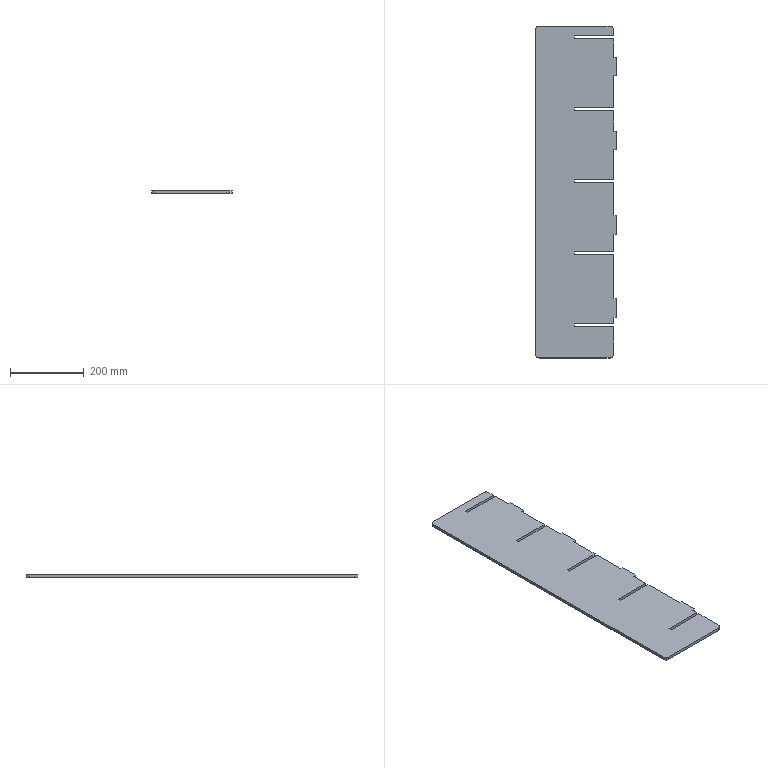Part | SolidWorks | features FlatPattern 1, SMBaseFlange 1, SheetMetal 1 | 1 solid | 46 faces | box 219.5 x 900 x 8 mm | volume 1503633 mm3 | plane 42 | cylinder 4 | commonest cylinder face diameters 20 x4
STEP:
#1=CARTESIAN_POINT('',(-1003.006,359.062,0.));
#2=VERTEX_POINT('',#1);
#3=CARTESIAN_POINT('',(-1013.006,369.062,0.));
#4=VERTEX_POINT('',#3);
#5=CARTESIAN_POINT('',(-1013.006,359.062,0.));
#6=DIRECTION('',(0.,0.,1.));
#7=DIRECTION('',(-1.,0.,0.));
#8=AXIS2_PLACEMENT_3D('',#5,#6,#7);
#9=CIRCLE('',#8,10.);
#10=EDGE_CURVE('',#2,#4,#9,.T.);
#11=ORIENTED_EDGE('',*,*,#10,.F.);
#12=CARTESIAN_POINT('',(-1003.006,359.062,-8.));
#13=VERTEX_POINT('',#12);
#14=CARTESIAN_POINT('',(-1003.006,359.062,-8.));
#15=DIRECTION('',(0.,0.,1.));
#16=VECTOR('',#15,1000.);
#17=LINE('',#14,#16);
#18=EDGE_CURVE('',#13,#2,#17,.T.);
#19=ORIENTED_EDGE('',*,*,#18,.F.);
#20=CARTESIAN_POINT('',(-1013.006,369.062,-8.));
#21=VERTEX_POINT('',#20);
#22=CARTESIAN_POINT('',(-1013.006,359.062,-8.));
#23=DIRECTION('',(0.,0.,1.));
#24=DIRECTION('',(-1.,0.,0.));
#25=AXIS2_PLACEMENT_3D('',#22,#23,#24);
#26=CIRCLE('',#25,10.);
#27=EDGE_CURVE('',#13,#21,#26,.T.);
#28=ORIENTED_EDGE('',*,*,#27,.T.);
#29=CARTESIAN_POINT('',(-1013.006,369.062,-8.));
#30=DIRECTION('',(0.,0.,1.));
#31=VECTOR('',#30,1000.);
#32=LINE('',#29,#31);
#33=EDGE_CURVE('',#21,#4,#32,.T.);
#34=ORIENTED_EDGE('',*,*,#33,.T.);
#35=EDGE_LOOP('',(#11,#19,#28,#34));
#36=FACE_OUTER_BOUND('',#35,.T.);
#37=CARTESIAN_POINT('',(-1013.006,359.062,-8.));
#38=DIRECTION('',(0.,0.,1.));
#39=DIRECTION('',(1.,0.,0.));
#40=AXIS2_PLACEMENT_3D('',#37,#38,#39);
#41=CYLINDRICAL_SURFACE('',#40,10.);
#42=ADVANCED_FACE('',(#36),#41,.T.);
#43=CARTESIAN_POINT('',(-1003.006,342.062,0.));
#44=VERTEX_POINT('',#43);
#45=CARTESIAN_POINT('',(-1003.006,359.062,0.));
#46=DIRECTION('',(0.,1.,0.));
#47=VECTOR('',#46,1000.);
#48=LINE('',#45,#47);
#49=EDGE_CURVE('',#44,#2,#48,.T.);
#50=ORIENTED_EDGE('',*,*,#49,.F.);
#51=CARTESIAN_POINT('',(-1003.006,342.062,-8.));
#52=VERTEX_POINT('',#51);
#53=CARTESIAN_POINT('',(-1003.006,342.062,-8.));
#54=DIRECTION('',(0.,0.,1.));
#55=VECTOR('',#54,1000.);
#56=LINE('',#53,#55);
#57=EDGE_CURVE('',#52,#44,#56,.T.);
#58=ORIENTED_EDGE('',*,*,#57,.F.);
#59=CARTESIAN_POINT('',(-1003.006,359.062,-8.));
#60=DIRECTION('',(0.,1.,0.));
#61=VECTOR('',#60,1000.);
#62=LINE('',#59,#61);
#63=EDGE_CURVE('',#52,#13,#62,.T.);
#64=ORIENTED_EDGE('',*,*,#63,.T.);
#65=ORIENTED_EDGE('',*,*,#18,.T.);
#66=EDGE_LOOP('',(#50,#58,#64,#65));
#67=FACE_OUTER_BOUND('',#66,.T.);
#68=CARTESIAN_POINT('',(-1003.006,359.062,-8.));
#69=DIRECTION('',(1.,0.,0.));
#70=DIRECTION('',(0.,0.,-1.));
#71=AXIS2_PLACEMENT_3D('',#68,#69,#70);
#72=PLANE('',#71);
#73=ADVANCED_FACE('',(#67),#72,.T.);
#74=CARTESIAN_POINT('',(-1109.506,342.062,0.));
#75=VERTEX_POINT('',#74);
#76=CARTESIAN_POINT('',(-1003.006,342.062,0.));
#77=DIRECTION('',(1.,0.,0.));
#78=VECTOR('',#77,1000.);
#79=LINE('',#76,#78);
#80=EDGE_CURVE('',#75,#44,#79,.T.);
#81=ORIENTED_EDGE('',*,*,#80,.F.);
#82=CARTESIAN_POINT('',(-1109.506,342.062,-8.));
#83=VERTEX_POINT('',#82);
#84=CARTESIAN_POINT('',(-1109.506,342.062,-8.));
#85=DIRECTION('',(0.,0.,1.));
#86=VECTOR('',#85,1000.);
#87=LINE('',#84,#86);
#88=EDGE_CURVE('',#83,#75,#87,.T.);
#89=ORIENTED_EDGE('',*,*,#88,.F.);
#90=CARTESIAN_POINT('',(-1003.006,342.062,-8.));
#91=DIRECTION('',(1.,0.,0.));
#92=VECTOR('',#91,1000.);
#93=LINE('',#90,#92);
#94=EDGE_CURVE('',#83,#52,#93,.T.);
#95=ORIENTED_EDGE('',*,*,#94,.T.);
#96=ORIENTED_EDGE('',*,*,#57,.T.);
#97=EDGE_LOOP('',(#81,#89,#95,#96));
#98=FACE_OUTER_BOUND('',#97,.T.);
#99=CARTESIAN_POINT('',(-1003.006,342.062,-8.));
#100=DIRECTION('',(0.,-1.,0.));
#101=DIRECTION('',(0.,0.,-1.));
#102=AXIS2_PLACEMENT_3D('',#99,#100,#101);
#103=PLANE('',#102);
#104=ADVANCED_FACE('',(#98),#103,.T.);
#105=CARTESIAN_POINT('',(-1109.506,334.062,0.));
#106=VERTEX_POINT('',#105);
#107=CARTESIAN_POINT('',(-1109.506,342.062,0.));
#108=DIRECTION('',(0.,1.,0.));
#109=VECTOR('',#108,1000.);
#110=LINE('',#107,#109);
#111=EDGE_CURVE('',#106,#75,#110,.T.);
#112=ORIENTED_EDGE('',*,*,#111,.F.);
#113=CARTESIAN_POINT('',(-1109.506,334.062,-8.));
#114=VERTEX_POINT('',#113);
#115=CARTESIAN_POINT('',(-1109.506,334.062,-8.));
#116=DIRECTION('',(0.,0.,1.));
#117=VECTOR('',#116,1000.);
#118=LINE('',#115,#117);
#119=EDGE_CURVE('',#114,#106,#118,.T.);
#120=ORIENTED_EDGE('',*,*,#119,.F.);
#121=CARTESIAN_POINT('',(-1109.506,342.062,-8.));
#122=DIRECTION('',(0.,1.,0.));
#123=VECTOR('',#122,1000.);
#124=LINE('',#121,#123);
#125=EDGE_CURVE('',#114,#83,#124,.T.);
#126=ORIENTED_EDGE('',*,*,#125,.T.);
#127=ORIENTED_EDGE('',*,*,#88,.T.);
#128=EDGE_LOOP('',(#112,#120,#126,#127));
#129=FACE_OUTER_BOUND('',#128,.T.);
#130=CARTESIAN_POINT('',(-1109.506,342.062,-8.));
#131=DIRECTION('',(1.,0.,0.));
#132=DIRECTION('',(0.,0.,-1.));
#133=AXIS2_PLACEMENT_3D('',#130,#131,#132);
#134=PLANE('',#133);
#135=ADVANCED_FACE('',(#129),#134,.T.);
#136=CARTESIAN_POINT('',(-1003.006,334.062,0.));
#137=VERTEX_POINT('',#136);
#138=CARTESIAN_POINT('',(-1109.506,334.062,0.));
#139=DIRECTION('',(-1.,0.,0.));
#140=VECTOR('',#139,1000.);
#141=LINE('',#138,#140);
#142=EDGE_CURVE('',#137,#106,#141,.T.);
#143=ORIENTED_EDGE('',*,*,#142,.F.);
#144=CARTESIAN_POINT('',(-1003.006,334.062,-8.));
#145=VERTEX_POINT('',#144);
#146=CARTESIAN_POINT('',(-1003.006,334.062,-8.));
#147=DIRECTION('',(0.,0.,1.));
#148=VECTOR('',#147,1000.);
#149=LINE('',#146,#148);
#150=EDGE_CURVE('',#145,#137,#149,.T.);
#151=ORIENTED_EDGE('',*,*,#150,.F.);
#152=CARTESIAN_POINT('',(-1109.506,334.062,-8.));
#153=DIRECTION('',(-1.,0.,0.));
#154=VECTOR('',#153,1000.);
#155=LINE('',#152,#154);
#156=EDGE_CURVE('',#145,#114,#155,.T.);
#157=ORIENTED_EDGE('',*,*,#156,.T.);
#158=ORIENTED_EDGE('',*,*,#119,.T.);
#159=EDGE_LOOP('',(#143,#151,#157,#158));
#160=FACE_OUTER_BOUND('',#159,.T.);
#161=CARTESIAN_POINT('',(-1109.506,334.062,-8.));
#162=DIRECTION('',(0.,1.,0.));
#163=DIRECTION('',(0.,0.,1.));
#164=AXIS2_PLACEMENT_3D('',#161,#162,#163);
#165=PLANE('',#164);
#166=ADVANCED_FACE('',(#160),#165,.T.);
#167=CARTESIAN_POINT('',(-1003.006,284.062,0.));
#168=VERTEX_POINT('',#167);
#169=CARTESIAN_POINT('',(-1003.006,334.062,0.));
#170=DIRECTION('',(0.,1.,0.));
#171=VECTOR('',#170,1000.);
#172=LINE('',#169,#171);
#173=EDGE_CURVE('',#168,#137,#172,.T.);
#174=ORIENTED_EDGE('',*,*,#173,.F.);
#175=CARTESIAN_POINT('',(-1003.006,284.062,-8.));
#176=VERTEX_POINT('',#175);
#177=CARTESIAN_POINT('',(-1003.006,284.062,-8.));
#178=DIRECTION('',(0.,0.,1.));
#179=VECTOR('',#178,1000.);
#180=LINE('',#177,#179);
#181=EDGE_CURVE('',#176,#168,#180,.T.);
#182=ORIENTED_EDGE('',*,*,#181,.F.);
#183=CARTESIAN_POINT('',(-1003.006,334.062,-8.));
#184=DIRECTION('',(0.,1.,0.));
#185=VECTOR('',#184,1000.);
#186=LINE('',#183,#185);
#187=EDGE_CURVE('',#176,#145,#186,.T.);
#188=ORIENTED_EDGE('',*,*,#187,.T.);
#189=ORIENTED_EDGE('',*,*,#150,.T.);
#190=EDGE_LOOP('',(#174,#182,#188,#189));
#191=FACE_OUTER_BOUND('',#190,.T.);
#192=CARTESIAN_POINT('',(-1003.006,334.062,-8.));
#193=DIRECTION('',(1.,0.,0.));
#194=DIRECTION('',(0.,0.,-1.));
#195=AXIS2_PLACEMENT_3D('',#192,#193,#194);
#196=PLANE('',#195);
#197=ADVANCED_FACE('',(#191),#196,.T.);
#198=CARTESIAN_POINT('',(-995.506,284.062,0.));
#199=VERTEX_POINT('',#198);
#200=CARTESIAN_POINT('',(-1003.006,284.062,0.));
#201=DIRECTION('',(-1.,0.,0.));
#202=VECTOR('',#201,1000.);
#203=LINE('',#200,#202);
#204=EDGE_CURVE('',#199,#168,#203,.T.);
#205=ORIENTED_EDGE('',*,*,#204,.F.);
#206=CARTESIAN_POINT('',(-995.506,284.062,-8.));
#207=VERTEX_POINT('',#206);
#208=CARTESIAN_POINT('',(-995.506,284.062,-8.));
#209=DIRECTION('',(0.,0.,1.));
#210=VECTOR('',#209,1000.);
#211=LINE('',#208,#210);
#212=EDGE_CURVE('',#207,#199,#211,.T.);
#213=ORIENTED_EDGE('',*,*,#212,.F.);
#214=CARTESIAN_POINT('',(-1003.006,284.062,-8.));
#215=DIRECTION('',(-1.,0.,0.));
#216=VECTOR('',#215,1000.);
#217=LINE('',#214,#216);
#218=EDGE_CURVE('',#207,#176,#217,.T.);
#219=ORIENTED_EDGE('',*,*,#218,.T.);
#220=ORIENTED_EDGE('',*,*,#181,.T.);
#221=EDGE_LOOP('',(#205,#213,#219,#220));
#222=FACE_OUTER_BOUND('',#221,.T.);
#223=CARTESIAN_POINT('',(-1003.006,284.062,-8.));
#224=DIRECTION('',(0.,1.,0.));
#225=DIRECTION('',(0.,0.,1.));
#226=AXIS2_PLACEMENT_3D('',#223,#224,#225);
#227=PLANE('',#226);
#228=ADVANCED_FACE('',(#222),#227,.T.);
#229=CARTESIAN_POINT('',(-995.506,234.062,0.));
#230=VERTEX_POINT('',#229);
#231=CARTESIAN_POINT('',(-995.506,284.062,0.));
#232=DIRECTION('',(0.,1.,0.));
#233=VECTOR('',#232,1000.);
#234=LINE('',#231,#233);
#235=EDGE_CURVE('',#230,#199,#234,.T.);
#236=ORIENTED_EDGE('',*,*,#235,.F.);
#237=CARTESIAN_POINT('',(-995.506,234.062,-8.));
#238=VERTEX_POINT('',#237);
#239=CARTESIAN_POINT('',(-995.506,234.062,-8.));
#240=DIRECTION('',(0.,0.,1.));
#241=VECTOR('',#240,1000.);
#242=LINE('',#239,#241);
#243=EDGE_CURVE('',#238,#230,#242,.T.);
#244=ORIENTED_EDGE('',*,*,#243,.F.);
#245=CARTESIAN_POINT('',(-995.506,284.062,-8.));
#246=DIRECTION('',(0.,1.,0.));
#247=VECTOR('',#246,1000.);
#248=LINE('',#245,#247);
#249=EDGE_CURVE('',#238,#207,#248,.T.);
#250=ORIENTED_EDGE('',*,*,#249,.T.);
#251=ORIENTED_EDGE('',*,*,#212,.T.);
#252=EDGE_LOOP('',(#236,#244,#250,#251));
#253=FACE_OUTER_BOUND('',#252,.T.);
#254=CARTESIAN_POINT('',(-995.506,284.062,-8.));
#255=DIRECTION('',(1.,0.,0.));
#256=DIRECTION('',(0.,0.,-1.));
#257=AXIS2_PLACEMENT_3D('',#254,#255,#256);
#258=PLANE('',#257);
#259=ADVANCED_FACE('',(#253),#258,.T.);
#260=CARTESIAN_POINT('',(-1003.006,234.062,0.));
#261=VERTEX_POINT('',#260);
#262=CARTESIAN_POINT('',(-995.506,234.062,0.));
#263=DIRECTION('',(1.,0.,0.));
#264=VECTOR('',#263,1000.);
#265=LINE('',#262,#264);
#266=EDGE_CURVE('',#261,#230,#265,.T.);
#267=ORIENTED_EDGE('',*,*,#266,.F.);
#268=CARTESIAN_POINT('',(-1003.006,234.062,-8.));
#269=VERTEX_POINT('',#268);
#270=CARTESIAN_POINT('',(-1003.006,234.062,-8.));
#271=DIRECTION('',(0.,0.,1.));
#272=VECTOR('',#271,1000.);
#273=LINE('',#270,#272);
#274=EDGE_CURVE('',#269,#261,#273,.T.);
#275=ORIENTED_EDGE('',*,*,#274,.F.);
#276=CARTESIAN_POINT('',(-995.506,234.062,-8.));
#277=DIRECTION('',(1.,0.,0.));
#278=VECTOR('',#277,1000.);
#279=LINE('',#276,#278);
#280=EDGE_CURVE('',#269,#238,#279,.T.);
#281=ORIENTED_EDGE('',*,*,#280,.T.);
#282=ORIENTED_EDGE('',*,*,#243,.T.);
#283=EDGE_LOOP('',(#267,#275,#281,#282));
#284=FACE_OUTER_BOUND('',#283,.T.);
#285=CARTESIAN_POINT('',(-995.506,234.062,-8.));
#286=DIRECTION('',(0.,-1.,0.));
#287=DIRECTION('',(0.,0.,-1.));
#288=AXIS2_PLACEMENT_3D('',#285,#286,#287);
#289=PLANE('',#288);
#290=ADVANCED_FACE('',(#284),#289,.T.);
#291=CARTESIAN_POINT('',(-1003.006,147.062,0.));
#292=VERTEX_POINT('',#291);
#293=CARTESIAN_POINT('',(-1003.006,234.062,0.));
#294=DIRECTION('',(0.,1.,0.));
#295=VECTOR('',#294,1000.);
#296=LINE('',#293,#295);
#297=EDGE_CURVE('',#292,#261,#296,.T.);
#298=ORIENTED_EDGE('',*,*,#297,.F.);
#299=CARTESIAN_POINT('',(-1003.006,147.062,-8.));
#300=VERTEX_POINT('',#299);
#301=CARTESIAN_POINT('',(-1003.006,147.062,-8.));
#302=DIRECTION('',(0.,0.,1.));
#303=VECTOR('',#302,1000.);
#304=LINE('',#301,#303);
#305=EDGE_CURVE('',#300,#292,#304,.T.);
#306=ORIENTED_EDGE('',*,*,#305,.F.);
#307=CARTESIAN_POINT('',(-1003.006,234.062,-8.));
#308=DIRECTION('',(0.,1.,0.));
#309=VECTOR('',#308,1000.);
#310=LINE('',#307,#309);
#311=EDGE_CURVE('',#300,#269,#310,.T.);
#312=ORIENTED_EDGE('',*,*,#311,.T.);
#313=ORIENTED_EDGE('',*,*,#274,.T.);
#314=EDGE_LOOP('',(#298,#306,#312,#313));
#315=FACE_OUTER_BOUND('',#314,.T.);
#316=CARTESIAN_POINT('',(-1003.006,234.062,-8.));
#317=DIRECTION('',(1.,0.,0.));
#318=DIRECTION('',(0.,0.,-1.));
#319=AXIS2_PLACEMENT_3D('',#316,#317,#318);
#320=PLANE('',#319);
#321=ADVANCED_FACE('',(#315),#320,.T.);
#322=CARTESIAN_POINT('',(-1109.506,147.062,0.));
#323=VERTEX_POINT('',#322);
#324=CARTESIAN_POINT('',(-1003.006,147.062,0.));
#325=DIRECTION('',(1.,0.,0.));
#326=VECTOR('',#325,1000.);
#327=LINE('',#324,#326);
#328=EDGE_CURVE('',#323,#292,#327,.T.);
#329=ORIENTED_EDGE('',*,*,#328,.F.);
#330=CARTESIAN_POINT('',(-1109.506,147.062,-8.));
#331=VERTEX_POINT('',#330);
#332=CARTESIAN_POINT('',(-1109.506,147.062,-8.));
#333=DIRECTION('',(0.,0.,1.));
#334=VECTOR('',#333,1000.);
#335=LINE('',#332,#334);
#336=EDGE_CURVE('',#331,#323,#335,.T.);
#337=ORIENTED_EDGE('',*,*,#336,.F.);
#338=CARTESIAN_POINT('',(-1003.006,147.062,-8.));
#339=DIRECTION('',(1.,0.,0.));
#340=VECTOR('',#339,1000.);
#341=LINE('',#338,#340);
#342=EDGE_CURVE('',#331,#300,#341,.T.);
#343=ORIENTED_EDGE('',*,*,#342,.T.);
#344=ORIENTED_EDGE('',*,*,#305,.T.);
#345=EDGE_LOOP('',(#329,#337,#343,#344));
#346=FACE_OUTER_BOUND('',#345,.T.);
#347=CARTESIAN_POINT('',(-1003.006,147.062,-8.));
#348=DIRECTION('',(0.,-1.,0.));
#349=DIRECTION('',(0.,0.,-1.));
#350=AXIS2_PLACEMENT_3D('',#347,#348,#349);
#351=PLANE('',#350);
#352=ADVANCED_FACE('',(#346),#351,.T.);
#353=CARTESIAN_POINT('',(-1109.506,139.062,0.));
#354=VERTEX_POINT('',#353);
#355=CARTESIAN_POINT('',(-1109.506,147.062,0.));
#356=DIRECTION('',(0.,1.,0.));
#357=VECTOR('',#356,1000.);
#358=LINE('',#355,#357);
#359=EDGE_CURVE('',#354,#323,#358,.T.);
#360=ORIENTED_EDGE('',*,*,#359,.F.);
#361=CARTESIAN_POINT('',(-1109.506,139.062,-8.));
#362=VERTEX_POINT('',#361);
#363=CARTESIAN_POINT('',(-1109.506,139.062,-8.));
#364=DIRECTION('',(0.,0.,1.));
#365=VECTOR('',#364,1000.);
#366=LINE('',#363,#365);
#367=EDGE_CURVE('',#362,#354,#366,.T.);
#368=ORIENTED_EDGE('',*,*,#367,.F.);
#369=CARTESIAN_POINT('',(-1109.506,147.062,-8.));
#370=DIRECTION('',(0.,1.,0.));
#371=VECTOR('',#370,1000.);
#372=LINE('',#369,#371);
#373=EDGE_CURVE('',#362,#331,#372,.T.);
#374=ORIENTED_EDGE('',*,*,#373,.T.);
#375=ORIENTED_EDGE('',*,*,#336,.T.);
#376=EDGE_LOOP('',(#360,#368,#374,#375));
#377=FACE_OUTER_BOUND('',#376,.T.);
#378=CARTESIAN_POINT('',(-1109.506,147.062,-8.));
#379=DIRECTION('',(1.,0.,0.));
#380=DIRECTION('',(0.,0.,-1.));
#381=AXIS2_PLACEMENT_3D('',#378,#379,#380);
#382=PLANE('',#381);
#383=ADVANCED_FACE('',(#377),#382,.T.);
#384=CARTESIAN_POINT('',(-1003.006,139.062,0.));
#385=VERTEX_POINT('',#384);
#386=CARTESIAN_POINT('',(-1109.506,139.062,0.));
#387=DIRECTION('',(-1.,0.,0.));
#388=VECTOR('',#387,1000.);
#389=LINE('',#386,#388);
#390=EDGE_CURVE('',#385,#354,#389,.T.);
#391=ORIENTED_EDGE('',*,*,#390,.F.);
#392=CARTESIAN_POINT('',(-1003.006,139.062,-8.));
#393=VERTEX_POINT('',#392);
#394=CARTESIAN_POINT('',(-1003.006,139.062,-8.));
#395=DIRECTION('',(0.,0.,1.));
#396=VECTOR('',#395,1000.);
#397=LINE('',#394,#396);
#398=EDGE_CURVE('',#393,#385,#397,.T.);
#399=ORIENTED_EDGE('',*,*,#398,.F.);
#400=CARTESIAN_POINT('',(-1109.506,139.062,-8.));
#401=DIRECTION('',(-1.,0.,0.));
#402=VECTOR('',#401,1000.);
#403=LINE('',#400,#402);
#404=EDGE_CURVE('',#393,#362,#403,.T.);
#405=ORIENTED_EDGE('',*,*,#404,.T.);
#406=ORIENTED_EDGE('',*,*,#367,.T.);
#407=EDGE_LOOP('',(#391,#399,#405,#406));
#408=FACE_OUTER_BOUND('',#407,.T.);
#409=CARTESIAN_POINT('',(-1109.506,139.062,-8.));
#410=DIRECTION('',(0.,1.,0.));
#411=DIRECTION('',(0.,0.,1.));
#412=AXIS2_PLACEMENT_3D('',#409,#410,#411);
#413=PLANE('',#412);
#414=ADVANCED_FACE('',(#408),#413,.T.);
#415=CARTESIAN_POINT('',(-1003.006,84.062,0.));
#416=VERTEX_POINT('',#415);
#417=CARTESIAN_POINT('',(-1003.006,139.062,0.));
#418=DIRECTION('',(0.,1.,0.));
#419=VECTOR('',#418,1000.);
#420=LINE('',#417,#419);
#421=EDGE_CURVE('',#416,#385,#420,.T.);
#422=ORIENTED_EDGE('',*,*,#421,.F.);
#423=CARTESIAN_POINT('',(-1003.006,84.062,-8.));
#424=VERTEX_POINT('',#423);
#425=CARTESIAN_POINT('',(-1003.006,84.062,-8.));
#426=DIRECTION('',(0.,0.,1.));
#427=VECTOR('',#426,1000.);
#428=LINE('',#425,#427);
#429=EDGE_CURVE('',#424,#416,#428,.T.);
#430=ORIENTED_EDGE('',*,*,#429,.F.);
#431=CARTESIAN_POINT('',(-1003.006,139.062,-8.));
#432=DIRECTION('',(0.,1.,0.));
#433=VECTOR('',#432,1000.);
#434=LINE('',#431,#433);
#435=EDGE_CURVE('',#424,#393,#434,.T.);
#436=ORIENTED_EDGE('',*,*,#435,.T.);
#437=ORIENTED_EDGE('',*,*,#398,.T.);
#438=EDGE_LOOP('',(#422,#430,#436,#437));
#439=FACE_OUTER_BOUND('',#438,.T.);
#440=CARTESIAN_POINT('',(-1003.006,139.062,-8.));
#441=DIRECTION('',(1.,0.,0.));
#442=DIRECTION('',(0.,0.,-1.));
#443=AXIS2_PLACEMENT_3D('',#440,#441,#442);
#444=PLANE('',#443);
#445=ADVANCED_FACE('',(#439),#444,.T.);
#446=CARTESIAN_POINT('',(-995.506,84.062,0.));
#447=VERTEX_POINT('',#446);
#448=CARTESIAN_POINT('',(-1003.006,84.062,0.));
#449=DIRECTION('',(-1.,0.,0.));
#450=VECTOR('',#449,1000.);
#451=LINE('',#448,#450);
#452=EDGE_CURVE('',#447,#416,#451,.T.);
#453=ORIENTED_EDGE('',*,*,#452,.F.);
#454=CARTESIAN_POINT('',(-995.506,84.062,-8.));
#455=VERTEX_POINT('',#454);
#456=CARTESIAN_POINT('',(-995.506,84.062,-8.));
#457=DIRECTION('',(0.,0.,1.));
#458=VECTOR('',#457,1000.);
#459=LINE('',#456,#458);
#460=EDGE_CURVE('',#455,#447,#459,.T.);
#461=ORIENTED_EDGE('',*,*,#460,.F.);
#462=CARTESIAN_POINT('',(-1003.006,84.062,-8.));
#463=DIRECTION('',(-1.,0.,0.));
#464=VECTOR('',#463,1000.);
#465=LINE('',#462,#464);
#466=EDGE_CURVE('',#455,#424,#465,.T.);
#467=ORIENTED_EDGE('',*,*,#466,.T.);
#468=ORIENTED_EDGE('',*,*,#429,.T.);
#469=EDGE_LOOP('',(#453,#461,#467,#468));
#470=FACE_OUTER_BOUND('',#469,.T.);
#471=CARTESIAN_POINT('',(-1003.006,84.062,-8.));
#472=DIRECTION('',(0.,1.,0.));
#473=DIRECTION('',(0.,0.,1.));
#474=AXIS2_PLACEMENT_3D('',#471,#472,#473);
#475=PLANE('',#474);
#476=ADVANCED_FACE('',(#470),#475,.T.);
#477=CARTESIAN_POINT('',(-995.506,34.062,0.));
#478=VERTEX_POINT('',#477);
#479=CARTESIAN_POINT('',(-995.506,84.062,0.));
#480=DIRECTION('',(0.,1.,0.));
#481=VECTOR('',#480,1000.);
#482=LINE('',#479,#481);
#483=EDGE_CURVE('',#478,#447,#482,.T.);
#484=ORIENTED_EDGE('',*,*,#483,.F.);
#485=CARTESIAN_POINT('',(-995.506,34.062,-8.));
#486=VERTEX_POINT('',#485);
#487=CARTESIAN_POINT('',(-995.506,34.062,-8.));
#488=DIRECTION('',(0.,0.,1.));
#489=VECTOR('',#488,1000.);
#490=LINE('',#487,#489);
#491=EDGE_CURVE('',#486,#478,#490,.T.);
#492=ORIENTED_EDGE('',*,*,#491,.F.);
#493=CARTESIAN_POINT('',(-995.506,84.062,-8.));
#494=DIRECTION('',(0.,1.,0.));
#495=VECTOR('',#494,1000.);
#496=LINE('',#493,#495);
#497=EDGE_CURVE('',#486,#455,#496,.T.);
#498=ORIENTED_EDGE('',*,*,#497,.T.);
#499=ORIENTED_EDGE('',*,*,#460,.T.);
#500=EDGE_LOOP('',(#484,#492,#498,#499));
#501=FACE_OUTER_BOUND('',#500,.T.);
#502=CARTESIAN_POINT('',(-995.506,84.062,-8.));
#503=DIRECTION('',(1.,0.,0.));
#504=DIRECTION('',(0.,0.,-1.));
#505=AXIS2_PLACEMENT_3D('',#502,#503,#504);
#506=PLANE('',#505);
#507=ADVANCED_FACE('',(#501),#506,.T.);
#508=CARTESIAN_POINT('',(-1003.006,34.062,0.));
#509=VERTEX_POINT('',#508);
#510=CARTESIAN_POINT('',(-995.506,34.062,0.));
#511=DIRECTION('',(1.,0.,0.));
#512=VECTOR('',#511,1000.);
#513=LINE('',#510,#512);
#514=EDGE_CURVE('',#509,#478,#513,.T.);
#515=ORIENTED_EDGE('',*,*,#514,.F.);
#516=CARTESIAN_POINT('',(-1003.006,34.062,-8.));
#517=VERTEX_POINT('',#516);
#518=CARTESIAN_POINT('',(-1003.006,34.062,-8.));
#519=DIRECTION('',(0.,0.,1.));
#520=VECTOR('',#519,1000.);
#521=LINE('',#518,#520);
#522=EDGE_CURVE('',#517,#509,#521,.T.);
#523=ORIENTED_EDGE('',*,*,#522,.F.);
#524=CARTESIAN_POINT('',(-995.506,34.062,-8.));
#525=DIRECTION('',(1.,0.,0.));
#526=VECTOR('',#525,1000.);
#527=LINE('',#524,#526);
#528=EDGE_CURVE('',#517,#486,#527,.T.);
#529=ORIENTED_EDGE('',*,*,#528,.T.);
#530=ORIENTED_EDGE('',*,*,#491,.T.);
#531=EDGE_LOOP('',(#515,#523,#529,#530));
#532=FACE_OUTER_BOUND('',#531,.T.);
#533=CARTESIAN_POINT('',(-995.506,34.062,-8.));
#534=DIRECTION('',(0.,-1.,0.));
#535=DIRECTION('',(1.,0.,0.));
#536=AXIS2_PLACEMENT_3D('',#533,#534,#535);
#537=PLANE('',#536);
#538=ADVANCED_FACE('',(#532),#537,.T.);
#539=CARTESIAN_POINT('',(-1003.006,-47.938,0.));
#540=VERTEX_POINT('',#539);
#541=CARTESIAN_POINT('',(-1003.006,34.062,0.));
#542=DIRECTION('',(0.,1.,0.));
#543=VECTOR('',#542,1000.);
#544=LINE('',#541,#543);
#545=EDGE_CURVE('',#540,#509,#544,.T.);
#546=ORIENTED_EDGE('',*,*,#545,.F.);
#547=CARTESIAN_POINT('',(-1003.006,-47.938,-8.));
#548=VERTEX_POINT('',#547);
#549=CARTESIAN_POINT('',(-1003.006,-47.938,-8.));
#550=DIRECTION('',(0.,0.,1.));
#551=VECTOR('',#550,1000.);
#552=LINE('',#549,#551);
#553=EDGE_CURVE('',#548,#540,#552,.T.);
#554=ORIENTED_EDGE('',*,*,#553,.F.);
#555=CARTESIAN_POINT('',(-1003.006,34.062,-8.));
#556=DIRECTION('',(0.,1.,0.));
#557=VECTOR('',#556,1000.);
#558=LINE('',#555,#557);
#559=EDGE_CURVE('',#548,#517,#558,.T.);
#560=ORIENTED_EDGE('',*,*,#559,.T.);
#561=ORIENTED_EDGE('',*,*,#522,.T.);
#562=EDGE_LOOP('',(#546,#554,#560,#561));
#563=FACE_OUTER_BOUND('',#562,.T.);
#564=CARTESIAN_POINT('',(-1003.006,34.062,-8.));
#565=DIRECTION('',(1.,0.,0.));
#566=DIRECTION('',(0.,0.,-1.));
#567=AXIS2_PLACEMENT_3D('',#564,#565,#566);
#568=PLANE('',#567);
#569=ADVANCED_FACE('',(#563),#568,.T.);
#570=CARTESIAN_POINT('',(-1109.506,-47.938,0.));
#571=VERTEX_POINT('',#570);
#572=CARTESIAN_POINT('',(-1003.006,-47.938,0.));
#573=DIRECTION('',(1.,0.,0.));
#574=VECTOR('',#573,1000.);
#575=LINE('',#572,#574);
#576=EDGE_CURVE('',#571,#540,#575,.T.);
#577=ORIENTED_EDGE('',*,*,#576,.F.);
#578=CARTESIAN_POINT('',(-1109.506,-47.938,-8.));
#579=VERTEX_POINT('',#578);
#580=CARTESIAN_POINT('',(-1109.506,-47.938,-8.));
#581=DIRECTION('',(0.,0.,1.));
#582=VECTOR('',#581,1000.);
#583=LINE('',#580,#582);
#584=EDGE_CURVE('',#579,#571,#583,.T.);
#585=ORIENTED_EDGE('',*,*,#584,.F.);
#586=CARTESIAN_POINT('',(-1003.006,-47.938,-8.));
#587=DIRECTION('',(1.,0.,0.));
#588=VECTOR('',#587,1000.);
#589=LINE('',#586,#588);
#590=EDGE_CURVE('',#579,#548,#589,.T.);
#591=ORIENTED_EDGE('',*,*,#590,.T.);
#592=ORIENTED_EDGE('',*,*,#553,.T.);
#593=EDGE_LOOP('',(#577,#585,#591,#592));
#594=FACE_OUTER_BOUND('',#593,.T.);
#595=CARTESIAN_POINT('',(-1003.006,-47.938,-8.));
#596=DIRECTION('',(0.,-1.,0.));
#597=DIRECTION('',(1.,0.,0.));
#598=AXIS2_PLACEMENT_3D('',#595,#596,#597);
#599=PLANE('',#598);
#600=ADVANCED_FACE('',(#594),#599,.T.);
#601=CARTESIAN_POINT('',(-1109.506,-55.938,0.));
#602=VERTEX_POINT('',#601);
#603=CARTESIAN_POINT('',(-1109.506,-47.938,0.));
#604=DIRECTION('',(0.,1.,0.));
#605=VECTOR('',#604,1000.);
#606=LINE('',#603,#605);
#607=EDGE_CURVE('',#602,#571,#606,.T.);
#608=ORIENTED_EDGE('',*,*,#607,.F.);
#609=CARTESIAN_POINT('',(-1109.506,-55.938,-8.));
#610=VERTEX_POINT('',#609);
#611=CARTESIAN_POINT('',(-1109.506,-55.938,-8.));
#612=DIRECTION('',(0.,0.,1.));
#613=VECTOR('',#612,1000.);
#614=LINE('',#611,#613);
#615=EDGE_CURVE('',#610,#602,#614,.T.);
#616=ORIENTED_EDGE('',*,*,#615,.F.);
#617=CARTESIAN_POINT('',(-1109.506,-47.938,-8.));
#618=DIRECTION('',(0.,1.,0.));
#619=VECTOR('',#618,1000.);
#620=LINE('',#617,#619);
#621=EDGE_CURVE('',#610,#579,#620,.T.);
#622=ORIENTED_EDGE('',*,*,#621,.T.);
#623=ORIENTED_EDGE('',*,*,#584,.T.);
#624=EDGE_LOOP('',(#608,#616,#622,#623));
#625=FACE_OUTER_BOUND('',#624,.T.);
#626=CARTESIAN_POINT('',(-1109.506,-47.938,-8.));
#627=DIRECTION('',(1.,0.,0.));
#628=DIRECTION('',(0.,0.,-1.));
#629=AXIS2_PLACEMENT_3D('',#626,#627,#628);
#630=PLANE('',#629);
#631=ADVANCED_FACE('',(#625),#630,.T.);
#632=CARTESIAN_POINT('',(-1003.006,-55.938,0.));
#633=VERTEX_POINT('',#632);
#634=CARTESIAN_POINT('',(-1109.506,-55.938,0.));
#635=DIRECTION('',(-1.,0.,0.));
#636=VECTOR('',#635,1000.);
#637=LINE('',#634,#636);
#638=EDGE_CURVE('',#633,#602,#637,.T.);
#639=ORIENTED_EDGE('',*,*,#638,.F.);
#640=CARTESIAN_POINT('',(-1003.006,-55.938,-8.));
#641=VERTEX_POINT('',#640);
#642=CARTESIAN_POINT('',(-1003.006,-55.938,-8.));
#643=DIRECTION('',(0.,0.,1.));
#644=VECTOR('',#643,1000.);
#645=LINE('',#642,#644);
#646=EDGE_CURVE('',#641,#633,#645,.T.);
#647=ORIENTED_EDGE('',*,*,#646,.F.);
#648=CARTESIAN_POINT('',(-1109.506,-55.938,-8.));
#649=DIRECTION('',(-1.,0.,0.));
#650=VECTOR('',#649,1000.);
#651=LINE('',#648,#650);
#652=EDGE_CURVE('',#641,#610,#651,.T.);
#653=ORIENTED_EDGE('',*,*,#652,.T.);
#654=ORIENTED_EDGE('',*,*,#615,.T.);
#655=EDGE_LOOP('',(#639,#647,#653,#654));
#656=FACE_OUTER_BOUND('',#655,.T.);
#657=CARTESIAN_POINT('',(-1109.506,-55.938,-8.));
#658=DIRECTION('',(0.,1.,0.));
#659=DIRECTION('',(-1.,0.,0.));
#660=AXIS2_PLACEMENT_3D('',#657,#658,#659);
#661=PLANE('',#660);
#662=ADVANCED_FACE('',(#656),#661,.T.);
#663=CARTESIAN_POINT('',(-1003.006,-145.938,0.));
#664=VERTEX_POINT('',#663);
#665=CARTESIAN_POINT('',(-1003.006,-55.938,0.));
#666=DIRECTION('',(0.,1.,0.));
#667=VECTOR('',#666,1000.);
#668=LINE('',#665,#667);
#669=EDGE_CURVE('',#664,#633,#668,.T.);
#670=ORIENTED_EDGE('',*,*,#669,.F.);
#671=CARTESIAN_POINT('',(-1003.006,-145.938,-8.));
#672=VERTEX_POINT('',#671);
#673=CARTESIAN_POINT('',(-1003.006,-145.938,-8.));
#674=DIRECTION('',(0.,0.,1.));
#675=VECTOR('',#674,1000.);
#676=LINE('',#673,#675);
#677=EDGE_CURVE('',#672,#664,#676,.T.);
#678=ORIENTED_EDGE('',*,*,#677,.F.);
#679=CARTESIAN_POINT('',(-1003.006,-55.938,-8.));
#680=DIRECTION('',(0.,1.,0.));
#681=VECTOR('',#680,1000.);
#682=LINE('',#679,#681);
#683=EDGE_CURVE('',#672,#641,#682,.T.);
#684=ORIENTED_EDGE('',*,*,#683,.T.);
#685=ORIENTED_EDGE('',*,*,#646,.T.);
#686=EDGE_LOOP('',(#670,#678,#684,#685));
#687=FACE_OUTER_BOUND('',#686,.T.);
#688=CARTESIAN_POINT('',(-1003.006,-55.938,-8.));
#689=DIRECTION('',(1.,0.,0.));
#690=DIRECTION('',(0.,0.,-1.));
#691=AXIS2_PLACEMENT_3D('',#688,#689,#690);
#692=PLANE('',#691);
#693=ADVANCED_FACE('',(#687),#692,.T.);
#694=CARTESIAN_POINT('',(-995.506,-145.938,0.));
#695=VERTEX_POINT('',#694);
#696=CARTESIAN_POINT('',(-1003.006,-145.938,0.));
#697=DIRECTION('',(-1.,0.,0.));
#698=VECTOR('',#697,1000.);
#699=LINE('',#696,#698);
#700=EDGE_CURVE('',#695,#664,#699,.T.);
#701=ORIENTED_EDGE('',*,*,#700,.F.);
#702=CARTESIAN_POINT('',(-995.506,-145.938,-8.));
#703=VERTEX_POINT('',#702);
#704=CARTESIAN_POINT('',(-995.506,-145.938,-8.));
#705=DIRECTION('',(0.,0.,1.));
#706=VECTOR('',#705,1000.);
#707=LINE('',#704,#706);
#708=EDGE_CURVE('',#703,#695,#707,.T.);
#709=ORIENTED_EDGE('',*,*,#708,.F.);
#710=CARTESIAN_POINT('',(-1003.006,-145.938,-8.));
#711=DIRECTION('',(-1.,0.,0.));
#712=VECTOR('',#711,1000.);
#713=LINE('',#710,#712);
#714=EDGE_CURVE('',#703,#672,#713,.T.);
#715=ORIENTED_EDGE('',*,*,#714,.T.);
#716=ORIENTED_EDGE('',*,*,#677,.T.);
#717=EDGE_LOOP('',(#701,#709,#715,#716));
#718=FACE_OUTER_BOUND('',#717,.T.);
#719=CARTESIAN_POINT('',(-1003.006,-145.938,-8.));
#720=DIRECTION('',(0.,1.,0.));
#721=DIRECTION('',(0.,0.,1.));
#722=AXIS2_PLACEMENT_3D('',#719,#720,#721);
#723=PLANE('',#722);
#724=ADVANCED_FACE('',(#718),#723,.T.);
#725=CARTESIAN_POINT('',(-995.506,-195.938,0.));
#726=VERTEX_POINT('',#725);
#727=CARTESIAN_POINT('',(-995.506,-145.938,0.));
#728=DIRECTION('',(0.,1.,0.));
#729=VECTOR('',#728,1000.);
#730=LINE('',#727,#729);
#731=EDGE_CURVE('',#726,#695,#730,.T.);
#732=ORIENTED_EDGE('',*,*,#731,.F.);
#733=CARTESIAN_POINT('',(-995.506,-195.938,-8.));
#734=VERTEX_POINT('',#733);
#735=CARTESIAN_POINT('',(-995.506,-195.938,-8.));
#736=DIRECTION('',(0.,0.,1.));
#737=VECTOR('',#736,1000.);
#738=LINE('',#735,#737);
#739=EDGE_CURVE('',#734,#726,#738,.T.);
#740=ORIENTED_EDGE('',*,*,#739,.F.);
#741=CARTESIAN_POINT('',(-995.506,-145.938,-8.));
#742=DIRECTION('',(0.,1.,0.));
#743=VECTOR('',#742,1000.);
#744=LINE('',#741,#743);
#745=EDGE_CURVE('',#734,#703,#744,.T.);
#746=ORIENTED_EDGE('',*,*,#745,.T.);
#747=ORIENTED_EDGE('',*,*,#708,.T.);
#748=EDGE_LOOP('',(#732,#740,#746,#747));
#749=FACE_OUTER_BOUND('',#748,.T.);
#750=CARTESIAN_POINT('',(-995.506,-145.938,-8.));
#751=DIRECTION('',(1.,0.,0.));
#752=DIRECTION('',(0.,0.,-1.));
#753=AXIS2_PLACEMENT_3D('',#750,#751,#752);
#754=PLANE('',#753);
#755=ADVANCED_FACE('',(#749),#754,.T.);
#756=CARTESIAN_POINT('',(-1003.006,-195.938,0.));
#757=VERTEX_POINT('',#756);
#758=CARTESIAN_POINT('',(-995.506,-195.938,0.));
#759=DIRECTION('',(1.,0.,0.));
#760=VECTOR('',#759,1000.);
#761=LINE('',#758,#760);
#762=EDGE_CURVE('',#757,#726,#761,.T.);
#763=ORIENTED_EDGE('',*,*,#762,.F.);
#764=CARTESIAN_POINT('',(-1003.006,-195.938,-8.));
#765=VERTEX_POINT('',#764);
#766=CARTESIAN_POINT('',(-1003.006,-195.938,-8.));
#767=DIRECTION('',(0.,0.,1.));
#768=VECTOR('',#767,1000.);
#769=LINE('',#766,#768);
#770=EDGE_CURVE('',#765,#757,#769,.T.);
#771=ORIENTED_EDGE('',*,*,#770,.F.);
#772=CARTESIAN_POINT('',(-995.506,-195.938,-8.));
#773=DIRECTION('',(1.,0.,0.));
#774=VECTOR('',#773,1000.);
#775=LINE('',#772,#774);
#776=EDGE_CURVE('',#765,#734,#775,.T.);
#777=ORIENTED_EDGE('',*,*,#776,.T.);
#778=ORIENTED_EDGE('',*,*,#739,.T.);
#779=EDGE_LOOP('',(#763,#771,#777,#778));
#780=FACE_OUTER_BOUND('',#779,.T.);
#781=CARTESIAN_POINT('',(-995.506,-195.938,-8.));
#782=DIRECTION('',(0.,-1.,0.));
#783=DIRECTION('',(1.,0.,0.));
#784=AXIS2_PLACEMENT_3D('',#781,#782,#783);
#785=PLANE('',#784);
#786=ADVANCED_FACE('',(#780),#785,.T.);
#787=CARTESIAN_POINT('',(-1003.006,-242.938,0.));
#788=VERTEX_POINT('',#787);
#789=CARTESIAN_POINT('',(-1003.006,-195.938,0.));
#790=DIRECTION('',(0.,1.,0.));
#791=VECTOR('',#790,1000.);
#792=LINE('',#789,#791);
#793=EDGE_CURVE('',#788,#757,#792,.T.);
#794=ORIENTED_EDGE('',*,*,#793,.F.);
#795=CARTESIAN_POINT('',(-1003.006,-242.938,-8.));
#796=VERTEX_POINT('',#795);
#797=CARTESIAN_POINT('',(-1003.006,-242.938,-8.));
#798=DIRECTION('',(0.,0.,1.));
#799=VECTOR('',#798,1000.);
#800=LINE('',#797,#799);
#801=EDGE_CURVE('',#796,#788,#800,.T.);
#802=ORIENTED_EDGE('',*,*,#801,.F.);
#803=CARTESIAN_POINT('',(-1003.006,-195.938,-8.));
#804=DIRECTION('',(0.,1.,0.));
#805=VECTOR('',#804,1000.);
#806=LINE('',#803,#805);
#807=EDGE_CURVE('',#796,#765,#806,.T.);
#808=ORIENTED_EDGE('',*,*,#807,.T.);
#809=ORIENTED_EDGE('',*,*,#770,.T.);
#810=EDGE_LOOP('',(#794,#802,#808,#809));
#811=FACE_OUTER_BOUND('',#810,.T.);
#812=CARTESIAN_POINT('',(-1003.006,-195.938,-8.));
#813=DIRECTION('',(1.,0.,0.));
#814=DIRECTION('',(0.,0.,-1.));
#815=AXIS2_PLACEMENT_3D('',#812,#813,#814);
#816=PLANE('',#815);
#817=ADVANCED_FACE('',(#811),#816,.T.);
#818=CARTESIAN_POINT('',(-1109.506,-242.938,0.));
#819=VERTEX_POINT('',#818);
#820=CARTESIAN_POINT('',(-1003.006,-242.938,0.));
#821=DIRECTION('',(1.,0.,0.));
#822=VECTOR('',#821,1000.);
#823=LINE('',#820,#822);
#824=EDGE_CURVE('',#819,#788,#823,.T.);
#825=ORIENTED_EDGE('',*,*,#824,.F.);
#826=CARTESIAN_POINT('',(-1109.506,-242.938,-8.));
#827=VERTEX_POINT('',#826);
#828=CARTESIAN_POINT('',(-1109.506,-242.938,-8.));
#829=DIRECTION('',(0.,0.,1.));
#830=VECTOR('',#829,1000.);
#831=LINE('',#828,#830);
#832=EDGE_CURVE('',#827,#819,#831,.T.);
#833=ORIENTED_EDGE('',*,*,#832,.F.);
#834=CARTESIAN_POINT('',(-1003.006,-242.938,-8.));
#835=DIRECTION('',(1.,0.,0.));
#836=VECTOR('',#835,1000.);
#837=LINE('',#834,#836);
#838=EDGE_CURVE('',#827,#796,#837,.T.);
#839=ORIENTED_EDGE('',*,*,#838,.T.);
#840=ORIENTED_EDGE('',*,*,#801,.T.);
#841=EDGE_LOOP('',(#825,#833,#839,#840));
#842=FACE_OUTER_BOUND('',#841,.T.);
#843=CARTESIAN_POINT('',(-1003.006,-242.938,-8.));
#844=DIRECTION('',(0.,-1.,0.));
#845=DIRECTION('',(0.,0.,-1.));
#846=AXIS2_PLACEMENT_3D('',#843,#844,#845);
#847=PLANE('',#846);
#848=ADVANCED_FACE('',(#842),#847,.T.);
#849=CARTESIAN_POINT('',(-1109.506,-250.938,0.));
#850=VERTEX_POINT('',#849);
#851=CARTESIAN_POINT('',(-1109.506,-242.938,0.));
#852=DIRECTION('',(0.,1.,0.));
#853=VECTOR('',#852,1000.);
#854=LINE('',#851,#853);
#855=EDGE_CURVE('',#850,#819,#854,.T.);
#856=ORIENTED_EDGE('',*,*,#855,.F.);
#857=CARTESIAN_POINT('',(-1109.506,-250.938,-8.));
#858=VERTEX_POINT('',#857);
#859=CARTESIAN_POINT('',(-1109.506,-250.938,-8.));
#860=DIRECTION('',(0.,0.,1.));
#861=VECTOR('',#860,1000.);
#862=LINE('',#859,#861);
#863=EDGE_CURVE('',#858,#850,#862,.T.);
#864=ORIENTED_EDGE('',*,*,#863,.F.);
#865=CARTESIAN_POINT('',(-1109.506,-242.938,-8.));
#866=DIRECTION('',(0.,1.,0.));
#867=VECTOR('',#866,1000.);
#868=LINE('',#865,#867);
#869=EDGE_CURVE('',#858,#827,#868,.T.);
#870=ORIENTED_EDGE('',*,*,#869,.T.);
#871=ORIENTED_EDGE('',*,*,#832,.T.);
#872=EDGE_LOOP('',(#856,#864,#870,#871));
#873=FACE_OUTER_BOUND('',#872,.T.);
#874=CARTESIAN_POINT('',(-1109.506,-242.938,-8.));
#875=DIRECTION('',(1.,0.,0.));
#876=DIRECTION('',(0.,0.,-1.));
#877=AXIS2_PLACEMENT_3D('',#874,#875,#876);
#878=PLANE('',#877);
#879=ADVANCED_FACE('',(#873),#878,.T.);
#880=CARTESIAN_POINT('',(-1003.006,-250.938,0.));
#881=VERTEX_POINT('',#880);
#882=CARTESIAN_POINT('',(-1109.506,-250.938,0.));
#883=DIRECTION('',(-1.,0.,0.));
#884=VECTOR('',#883,1000.);
#885=LINE('',#882,#884);
#886=EDGE_CURVE('',#881,#850,#885,.T.);
#887=ORIENTED_EDGE('',*,*,#886,.F.);
#888=CARTESIAN_POINT('',(-1003.006,-250.938,-8.));
#889=VERTEX_POINT('',#888);
#890=CARTESIAN_POINT('',(-1003.006,-250.938,-8.));
#891=DIRECTION('',(0.,0.,1.));
#892=VECTOR('',#891,1000.);
#893=LINE('',#890,#892);
#894=EDGE_CURVE('',#889,#881,#893,.T.);
#895=ORIENTED_EDGE('',*,*,#894,.F.);
#896=CARTESIAN_POINT('',(-1109.506,-250.938,-8.));
#897=DIRECTION('',(-1.,0.,0.));
#898=VECTOR('',#897,1000.);
#899=LINE('',#896,#898);
#900=EDGE_CURVE('',#889,#858,#899,.T.);
#901=ORIENTED_EDGE('',*,*,#900,.T.);
#902=ORIENTED_EDGE('',*,*,#863,.T.);
#903=EDGE_LOOP('',(#887,#895,#901,#902));
#904=FACE_OUTER_BOUND('',#903,.T.);
#905=CARTESIAN_POINT('',(-1109.506,-250.938,-8.));
#906=DIRECTION('',(0.,1.,0.));
#907=DIRECTION('',(0.,0.,1.));
#908=AXIS2_PLACEMENT_3D('',#905,#906,#907);
#909=PLANE('',#908);
#910=ADVANCED_FACE('',(#904),#909,.T.);
#911=CARTESIAN_POINT('',(-1003.006,-370.938,0.));
#912=VERTEX_POINT('',#911);
#913=CARTESIAN_POINT('',(-1003.006,-250.938,0.));
#914=DIRECTION('',(0.,1.,0.));
#915=VECTOR('',#914,1000.);
#916=LINE('',#913,#915);
#917=EDGE_CURVE('',#912,#881,#916,.T.);
#918=ORIENTED_EDGE('',*,*,#917,.F.);
#919=CARTESIAN_POINT('',(-1003.006,-370.938,-8.));
#920=VERTEX_POINT('',#919);
#921=CARTESIAN_POINT('',(-1003.006,-370.938,-8.));
#922=DIRECTION('',(0.,0.,1.));
#923=VECTOR('',#922,1000.);
#924=LINE('',#921,#923);
#925=EDGE_CURVE('',#920,#912,#924,.T.);
#926=ORIENTED_EDGE('',*,*,#925,.F.);
#927=CARTESIAN_POINT('',(-1003.006,-250.938,-8.));
#928=DIRECTION('',(0.,1.,0.));
#929=VECTOR('',#928,1000.);
#930=LINE('',#927,#929);
#931=EDGE_CURVE('',#920,#889,#930,.T.);
#932=ORIENTED_EDGE('',*,*,#931,.T.);
#933=ORIENTED_EDGE('',*,*,#894,.T.);
#934=EDGE_LOOP('',(#918,#926,#932,#933));
#935=FACE_OUTER_BOUND('',#934,.T.);
#936=CARTESIAN_POINT('',(-1003.006,-250.938,-8.));
#937=DIRECTION('',(1.,0.,0.));
#938=DIRECTION('',(0.,0.,-1.));
#939=AXIS2_PLACEMENT_3D('',#936,#937,#938);
#940=PLANE('',#939);
#941=ADVANCED_FACE('',(#935),#940,.T.);
#942=CARTESIAN_POINT('',(-995.506,-370.938,0.));
#943=VERTEX_POINT('',#942);
#944=CARTESIAN_POINT('',(-995.506,-370.938,0.));
#945=DIRECTION('',(-1.,0.,0.));
#946=VECTOR('',#945,1000.);
#947=LINE('',#944,#946);
#948=EDGE_CURVE('',#943,#912,#947,.T.);
#949=ORIENTED_EDGE('',*,*,#948,.F.);
#950=CARTESIAN_POINT('',(-995.506,-370.938,-8.));
#951=VERTEX_POINT('',#950);
#952=CARTESIAN_POINT('',(-995.506,-370.938,-8.));
#953=DIRECTION('',(0.,0.,1.));
#954=VECTOR('',#953,1000.);
#955=LINE('',#952,#954);
#956=EDGE_CURVE('',#951,#943,#955,.T.);
#957=ORIENTED_EDGE('',*,*,#956,.F.);
#958=CARTESIAN_POINT('',(-995.506,-370.938,-8.));
#959=DIRECTION('',(-1.,0.,0.));
#960=VECTOR('',#959,1000.);
#961=LINE('',#958,#960);
#962=EDGE_CURVE('',#951,#920,#961,.T.);
#963=ORIENTED_EDGE('',*,*,#962,.T.);
#964=ORIENTED_EDGE('',*,*,#925,.T.);
#965=EDGE_LOOP('',(#949,#957,#963,#964));
#966=FACE_OUTER_BOUND('',#965,.T.);
#967=CARTESIAN_POINT('',(-995.506,-370.938,-8.));
#968=DIRECTION('',(0.,1.,0.));
#969=DIRECTION('',(0.,0.,1.));
#970=AXIS2_PLACEMENT_3D('',#967,#968,#969);
#971=PLANE('',#970);
#972=ADVANCED_FACE('',(#966),#971,.T.);
#973=CARTESIAN_POINT('',(-995.506,-420.938,0.));
#974=VERTEX_POINT('',#973);
#975=CARTESIAN_POINT('',(-995.506,-420.938,0.));
#976=DIRECTION('',(0.,1.,0.));
#977=VECTOR('',#976,1000.);
#978=LINE('',#975,#977);
#979=EDGE_CURVE('',#974,#943,#978,.T.);
#980=ORIENTED_EDGE('',*,*,#979,.F.);
#981=CARTESIAN_POINT('',(-995.506,-420.938,-8.));
#982=VERTEX_POINT('',#981);
#983=CARTESIAN_POINT('',(-995.506,-420.938,-8.));
#984=DIRECTION('',(0.,0.,1.));
#985=VECTOR('',#984,1000.);
#986=LINE('',#983,#985);
#987=EDGE_CURVE('',#982,#974,#986,.T.);
#988=ORIENTED_EDGE('',*,*,#987,.F.);
#989=CARTESIAN_POINT('',(-995.506,-420.938,-8.));
#990=DIRECTION('',(0.,1.,0.));
#991=VECTOR('',#990,1000.);
#992=LINE('',#989,#991);
#993=EDGE_CURVE('',#982,#951,#992,.T.);
#994=ORIENTED_EDGE('',*,*,#993,.T.);
#995=ORIENTED_EDGE('',*,*,#956,.T.);
#996=EDGE_LOOP('',(#980,#988,#994,#995));
#997=FACE_OUTER_BOUND('',#996,.T.);
#998=CARTESIAN_POINT('',(-995.506,-420.938,-8.));
#999=DIRECTION('',(1.,0.,0.));
#1000=DIRECTION('',(0.,0.,-1.));
#1001=AXIS2_PLACEMENT_3D('',#998,#999,#1000);
#1002=PLANE('',#1001);
#1003=ADVANCED_FACE('',(#997),#1002,.T.);
#1004=CARTESIAN_POINT('',(-1003.006,-420.938,0.));
#1005=VERTEX_POINT('',#1004);
#1006=CARTESIAN_POINT('',(-1003.006,-420.938,0.));
#1007=DIRECTION('',(1.,0.,0.));
#1008=VECTOR('',#1007,1000.);
#1009=LINE('',#1006,#1008);
#1010=EDGE_CURVE('',#1005,#974,#1009,.T.);
#1011=ORIENTED_EDGE('',*,*,#1010,.F.);
#1012=CARTESIAN_POINT('',(-1003.006,-420.938,-8.));
#1013=VERTEX_POINT('',#1012);
#1014=CARTESIAN_POINT('',(-1003.006,-420.938,-8.));
#1015=DIRECTION('',(0.,0.,1.));
#1016=VECTOR('',#1015,1000.);
#1017=LINE('',#1014,#1016);
#1018=EDGE_CURVE('',#1013,#1005,#1017,.T.);
#1019=ORIENTED_EDGE('',*,*,#1018,.F.);
#1020=CARTESIAN_POINT('',(-1003.006,-420.938,-8.));
#1021=DIRECTION('',(1.,0.,0.));
#1022=VECTOR('',#1021,1000.);
#1023=LINE('',#1020,#1022);
#1024=EDGE_CURVE('',#1013,#982,#1023,.T.);
#1025=ORIENTED_EDGE('',*,*,#1024,.T.);
#1026=ORIENTED_EDGE('',*,*,#987,.T.);
#1027=EDGE_LOOP('',(#1011,#1019,#1025,#1026));
#1028=FACE_OUTER_BOUND('',#1027,.T.);
#1029=CARTESIAN_POINT('',(-1003.006,-420.938,-8.));
#1030=DIRECTION('',(0.,-1.,0.));
#1031=DIRECTION('',(0.,0.,-1.));
#1032=AXIS2_PLACEMENT_3D('',#1029,#1030,#1031);
#1033=PLANE('',#1032);
#1034=ADVANCED_FACE('',(#1028),#1033,.T.);
#1035=CARTESIAN_POINT('',(-1003.006,-437.938,0.));
#1036=VERTEX_POINT('',#1035);
#1037=CARTESIAN_POINT('',(-1003.006,-420.938,0.));
#1038=DIRECTION('',(0.,1.,0.));
#1039=VECTOR('',#1038,1000.);
#1040=LINE('',#1037,#1039);
#1041=EDGE_CURVE('',#1036,#1005,#1040,.T.);
#1042=ORIENTED_EDGE('',*,*,#1041,.F.);
#1043=CARTESIAN_POINT('',(-1003.006,-437.938,-8.));
#1044=VERTEX_POINT('',#1043);
#1045=CARTESIAN_POINT('',(-1003.006,-437.938,-8.));
#1046=DIRECTION('',(0.,0.,1.));
#1047=VECTOR('',#1046,1000.);
#1048=LINE('',#1045,#1047);
#1049=EDGE_CURVE('',#1044,#1036,#1048,.T.);
#1050=ORIENTED_EDGE('',*,*,#1049,.F.);
#1051=CARTESIAN_POINT('',(-1003.006,-420.938,-8.));
#1052=DIRECTION('',(0.,1.,0.));
#1053=VECTOR('',#1052,1000.);
#1054=LINE('',#1051,#1053);
#1055=EDGE_CURVE('',#1044,#1013,#1054,.T.);
#1056=ORIENTED_EDGE('',*,*,#1055,.T.);
#1057=ORIENTED_EDGE('',*,*,#1018,.T.);
#1058=EDGE_LOOP('',(#1042,#1050,#1056,#1057));
#1059=FACE_OUTER_BOUND('',#1058,.T.);
#1060=CARTESIAN_POINT('',(-1003.006,-420.938,-8.));
#1061=DIRECTION('',(1.,0.,0.));
#1062=DIRECTION('',(0.,0.,-1.));
#1063=AXIS2_PLACEMENT_3D('',#1060,#1061,#1062);
#1064=PLANE('',#1063);
#1065=ADVANCED_FACE('',(#1059),#1064,.T.);
#1066=CARTESIAN_POINT('',(-1109.506,-437.938,0.));
#1067=VERTEX_POINT('',#1066);
#1068=CARTESIAN_POINT('',(-1003.006,-437.938,0.));
#1069=DIRECTION('',(1.,0.,0.));
#1070=VECTOR('',#1069,1000.);
#1071=LINE('',#1068,#1070);
#1072=EDGE_CURVE('',#1067,#1036,#1071,.T.);
#1073=ORIENTED_EDGE('',*,*,#1072,.F.);
#1074=CARTESIAN_POINT('',(-1109.506,-437.938,-8.));
#1075=VERTEX_POINT('',#1074);
#1076=CARTESIAN_POINT('',(-1109.506,-437.938,-8.));
#1077=DIRECTION('',(0.,0.,1.));
#1078=VECTOR('',#1077,1000.);
#1079=LINE('',#1076,#1078);
#1080=EDGE_CURVE('',#1075,#1067,#1079,.T.);
#1081=ORIENTED_EDGE('',*,*,#1080,.F.);
#1082=CARTESIAN_POINT('',(-1003.006,-437.938,-8.));
#1083=DIRECTION('',(1.,0.,0.));
#1084=VECTOR('',#1083,1000.);
#1085=LINE('',#1082,#1084);
#1086=EDGE_CURVE('',#1075,#1044,#1085,.T.);
#1087=ORIENTED_EDGE('',*,*,#1086,.T.);
#1088=ORIENTED_EDGE('',*,*,#1049,.T.);
#1089=EDGE_LOOP('',(#1073,#1081,#1087,#1088));
#1090=FACE_OUTER_BOUND('',#1089,.T.);
#1091=CARTESIAN_POINT('',(-1003.006,-437.938,-8.));
#1092=DIRECTION('',(0.,-1.,0.));
#1093=DIRECTION('',(0.,0.,-1.));
#1094=AXIS2_PLACEMENT_3D('',#1091,#1092,#1093);
#1095=PLANE('',#1094);
#1096=ADVANCED_FACE('',(#1090),#1095,.T.);
#1097=CARTESIAN_POINT('',(-1109.506,-445.938,0.));
#1098=VERTEX_POINT('',#1097);
#1099=CARTESIAN_POINT('',(-1109.506,-437.938,0.));
#1100=DIRECTION('',(0.,1.,0.));
#1101=VECTOR('',#1100,1000.);
#1102=LINE('',#1099,#1101);
#1103=EDGE_CURVE('',#1098,#1067,#1102,.T.);
#1104=ORIENTED_EDGE('',*,*,#1103,.F.);
#1105=CARTESIAN_POINT('',(-1109.506,-445.938,-8.));
#1106=VERTEX_POINT('',#1105);
#1107=CARTESIAN_POINT('',(-1109.506,-445.938,-8.));
#1108=DIRECTION('',(0.,0.,1.));
#1109=VECTOR('',#1108,1000.);
#1110=LINE('',#1107,#1109);
#1111=EDGE_CURVE('',#1106,#1098,#1110,.T.);
#1112=ORIENTED_EDGE('',*,*,#1111,.F.);
#1113=CARTESIAN_POINT('',(-1109.506,-437.938,-8.));
#1114=DIRECTION('',(0.,1.,0.));
#1115=VECTOR('',#1114,1000.);
#1116=LINE('',#1113,#1115);
#1117=EDGE_CURVE('',#1106,#1075,#1116,.T.);
#1118=ORIENTED_EDGE('',*,*,#1117,.T.);
#1119=ORIENTED_EDGE('',*,*,#1080,.T.);
#1120=EDGE_LOOP('',(#1104,#1112,#1118,#1119));
#1121=FACE_OUTER_BOUND('',#1120,.T.);
#1122=CARTESIAN_POINT('',(-1109.506,-437.938,-8.));
#1123=DIRECTION('',(1.,0.,0.));
#1124=DIRECTION('',(0.,0.,-1.));
#1125=AXIS2_PLACEMENT_3D('',#1122,#1123,#1124);
#1126=PLANE('',#1125);
#1127=ADVANCED_FACE('',(#1121),#1126,.T.);
#1128=CARTESIAN_POINT('',(-1003.006,-445.938,0.));
#1129=VERTEX_POINT('',#1128);
#1130=CARTESIAN_POINT('',(-1109.506,-445.938,0.));
#1131=DIRECTION('',(-1.,0.,0.));
#1132=VECTOR('',#1131,1000.);
#1133=LINE('',#1130,#1132);
#1134=EDGE_CURVE('',#1129,#1098,#1133,.T.);
#1135=ORIENTED_EDGE('',*,*,#1134,.F.);
#1136=CARTESIAN_POINT('',(-1003.006,-445.938,-8.));
#1137=VERTEX_POINT('',#1136);
#1138=CARTESIAN_POINT('',(-1003.006,-445.938,-8.));
#1139=DIRECTION('',(0.,0.,1.));
#1140=VECTOR('',#1139,1000.);
#1141=LINE('',#1138,#1140);
#1142=EDGE_CURVE('',#1137,#1129,#1141,.T.);
#1143=ORIENTED_EDGE('',*,*,#1142,.F.);
#1144=CARTESIAN_POINT('',(-1109.506,-445.938,-8.));
#1145=DIRECTION('',(-1.,0.,0.));
#1146=VECTOR('',#1145,1000.);
#1147=LINE('',#1144,#1146);
#1148=EDGE_CURVE('',#1137,#1106,#1147,.T.);
#1149=ORIENTED_EDGE('',*,*,#1148,.T.);
#1150=ORIENTED_EDGE('',*,*,#1111,.T.);
#1151=EDGE_LOOP('',(#1135,#1143,#1149,#1150));
#1152=FACE_OUTER_BOUND('',#1151,.T.);
#1153=CARTESIAN_POINT('',(-1109.506,-445.938,-8.));
#1154=DIRECTION('',(0.,1.,0.));
#1155=DIRECTION('',(0.,0.,1.));
#1156=AXIS2_PLACEMENT_3D('',#1153,#1154,#1155);
#1157=PLANE('',#1156);
#1158=ADVANCED_FACE('',(#1152),#1157,.T.);
#1159=CARTESIAN_POINT('',(-1003.006,-520.938,0.));
#1160=VERTEX_POINT('',#1159);
#1161=CARTESIAN_POINT('',(-1003.006,-445.938,0.));
#1162=DIRECTION('',(0.,1.,0.));
#1163=VECTOR('',#1162,1000.);
#1164=LINE('',#1161,#1163);
#1165=EDGE_CURVE('',#1160,#1129,#1164,.T.);
#1166=ORIENTED_EDGE('',*,*,#1165,.F.);
#1167=CARTESIAN_POINT('',(-1003.006,-520.938,-8.));
#1168=VERTEX_POINT('',#1167);
#1169=CARTESIAN_POINT('',(-1003.006,-520.938,-8.));
#1170=DIRECTION('',(0.,0.,1.));
#1171=VECTOR('',#1170,1000.);
#1172=LINE('',#1169,#1171);
#1173=EDGE_CURVE('',#1168,#1160,#1172,.T.);
#1174=ORIENTED_EDGE('',*,*,#1173,.F.);
#1175=CARTESIAN_POINT('',(-1003.006,-445.938,-8.));
#1176=DIRECTION('',(0.,1.,0.));
#1177=VECTOR('',#1176,1000.);
#1178=LINE('',#1175,#1177);
#1179=EDGE_CURVE('',#1168,#1137,#1178,.T.);
#1180=ORIENTED_EDGE('',*,*,#1179,.T.);
#1181=ORIENTED_EDGE('',*,*,#1142,.T.);
#1182=EDGE_LOOP('',(#1166,#1174,#1180,#1181));
#1183=FACE_OUTER_BOUND('',#1182,.T.);
#1184=CARTESIAN_POINT('',(-1003.006,-445.938,-8.));
#1185=DIRECTION('',(1.,0.,0.));
#1186=DIRECTION('',(0.,1.,0.));
#1187=AXIS2_PLACEMENT_3D('',#1184,#1185,#1186);
#1188=PLANE('',#1187);
#1189=ADVANCED_FACE('',(#1183),#1188,.T.);
#1190=CARTESIAN_POINT('',(-1013.006,-530.938,0.));
#1191=VERTEX_POINT('',#1190);
#1192=CARTESIAN_POINT('',(-1013.006,-520.938,0.));
#1193=DIRECTION('',(0.,0.,1.));
#1194=DIRECTION('',(-1.,0.,0.));
#1195=AXIS2_PLACEMENT_3D('',#1192,#1193,#1194);
#1196=CIRCLE('',#1195,10.);
#1197=EDGE_CURVE('',#1191,#1160,#1196,.T.);
#1198=ORIENTED_EDGE('',*,*,#1197,.F.);
#1199=CARTESIAN_POINT('',(-1013.006,-530.938,-8.));
#1200=VERTEX_POINT('',#1199);
#1201=CARTESIAN_POINT('',(-1013.006,-530.938,-8.));
#1202=DIRECTION('',(0.,0.,1.));
#1203=VECTOR('',#1202,1000.);
#1204=LINE('',#1201,#1203);
#1205=EDGE_CURVE('',#1200,#1191,#1204,.T.);
#1206=ORIENTED_EDGE('',*,*,#1205,.F.);
#1207=CARTESIAN_POINT('',(-1013.006,-520.938,-8.));
#1208=DIRECTION('',(0.,0.,1.));
#1209=DIRECTION('',(-1.,0.,0.));
#1210=AXIS2_PLACEMENT_3D('',#1207,#1208,#1209);
#1211=CIRCLE('',#1210,10.);
#1212=EDGE_CURVE('',#1200,#1168,#1211,.T.);
#1213=ORIENTED_EDGE('',*,*,#1212,.T.);
#1214=ORIENTED_EDGE('',*,*,#1173,.T.);
#1215=EDGE_LOOP('',(#1198,#1206,#1213,#1214));
#1216=FACE_OUTER_BOUND('',#1215,.T.);
#1217=CARTESIAN_POINT('',(-1013.006,-520.938,-8.));
#1218=DIRECTION('',(0.,0.,1.));
#1219=DIRECTION('',(1.,0.,0.));
#1220=AXIS2_PLACEMENT_3D('',#1217,#1218,#1219);
#1221=CYLINDRICAL_SURFACE('',#1220,10.);
#1222=ADVANCED_FACE('',(#1216),#1221,.T.);
#1223=CARTESIAN_POINT('',(-1205.006,-530.938,0.));
#1224=VERTEX_POINT('',#1223);
#1225=CARTESIAN_POINT('',(-1013.006,-530.938,0.));
#1226=DIRECTION('',(1.,0.,0.));
#1227=VECTOR('',#1226,1000.);
#1228=LINE('',#1225,#1227);
#1229=EDGE_CURVE('',#1224,#1191,#1228,.T.);
#1230=ORIENTED_EDGE('',*,*,#1229,.F.);
#1231=CARTESIAN_POINT('',(-1205.006,-530.938,-8.));
#1232=VERTEX_POINT('',#1231);
#1233=CARTESIAN_POINT('',(-1205.006,-530.938,-8.));
#1234=DIRECTION('',(0.,0.,1.));
#1235=VECTOR('',#1234,1000.);
#1236=LINE('',#1233,#1235);
#1237=EDGE_CURVE('',#1232,#1224,#1236,.T.);
#1238=ORIENTED_EDGE('',*,*,#1237,.F.);
#1239=CARTESIAN_POINT('',(-1013.006,-530.938,-8.));
#1240=DIRECTION('',(1.,0.,0.));
#1241=VECTOR('',#1240,1000.);
#1242=LINE('',#1239,#1241);
#1243=EDGE_CURVE('',#1232,#1200,#1242,.T.);
#1244=ORIENTED_EDGE('',*,*,#1243,.T.);
#1245=ORIENTED_EDGE('',*,*,#1205,.T.);
#1246=EDGE_LOOP('',(#1230,#1238,#1244,#1245));
#1247=FACE_OUTER_BOUND('',#1246,.T.);
#1248=CARTESIAN_POINT('',(-1013.006,-530.938,-8.));
#1249=DIRECTION('',(0.,-1.,0.));
#1250=DIRECTION('',(0.,0.,-1.));
#1251=AXIS2_PLACEMENT_3D('',#1248,#1249,#1250);
#1252=PLANE('',#1251);
#1253=ADVANCED_FACE('',(#1247),#1252,.T.);
#1254=CARTESIAN_POINT('',(-1215.006,-520.938,0.));
#1255=VERTEX_POINT('',#1254);
#1256=CARTESIAN_POINT('',(-1205.006,-520.938,0.));
#1257=DIRECTION('',(0.,0.,1.));
#1258=DIRECTION('',(-1.,0.,0.));
#1259=AXIS2_PLACEMENT_3D('',#1256,#1257,#1258);
#1260=CIRCLE('',#1259,10.);
#1261=EDGE_CURVE('',#1255,#1224,#1260,.T.);
#1262=ORIENTED_EDGE('',*,*,#1261,.F.);
#1263=CARTESIAN_POINT('',(-1215.006,-520.938,-8.));
#1264=VERTEX_POINT('',#1263);
#1265=CARTESIAN_POINT('',(-1215.006,-520.938,-8.));
#1266=DIRECTION('',(0.,0.,1.));
#1267=VECTOR('',#1266,1000.);
#1268=LINE('',#1265,#1267);
#1269=EDGE_CURVE('',#1264,#1255,#1268,.T.);
#1270=ORIENTED_EDGE('',*,*,#1269,.F.);
#1271=CARTESIAN_POINT('',(-1205.006,-520.938,-8.));
#1272=DIRECTION('',(0.,0.,1.));
#1273=DIRECTION('',(-1.,0.,0.));
#1274=AXIS2_PLACEMENT_3D('',#1271,#1272,#1273);
#1275=CIRCLE('',#1274,10.);
#1276=EDGE_CURVE('',#1264,#1232,#1275,.T.);
#1277=ORIENTED_EDGE('',*,*,#1276,.T.);
#1278=ORIENTED_EDGE('',*,*,#1237,.T.);
#1279=EDGE_LOOP('',(#1262,#1270,#1277,#1278));
#1280=FACE_OUTER_BOUND('',#1279,.T.);
#1281=CARTESIAN_POINT('',(-1205.006,-520.938,-8.));
#1282=DIRECTION('',(0.,0.,1.));
#1283=DIRECTION('',(1.,0.,0.));
#1284=AXIS2_PLACEMENT_3D('',#1281,#1282,#1283);
#1285=CYLINDRICAL_SURFACE('',#1284,10.);
#1286=ADVANCED_FACE('',(#1280),#1285,.T.);
#1287=CARTESIAN_POINT('',(-1215.006,359.062,0.));
#1288=VERTEX_POINT('',#1287);
#1289=CARTESIAN_POINT('',(-1215.006,359.062,0.));
#1290=DIRECTION('',(0.,-1.,0.));
#1291=VECTOR('',#1290,1000.);
#1292=LINE('',#1289,#1291);
#1293=EDGE_CURVE('',#1288,#1255,#1292,.T.);
#1294=ORIENTED_EDGE('',*,*,#1293,.F.);
#1295=CARTESIAN_POINT('',(-1215.006,359.062,-8.));
#1296=VERTEX_POINT('',#1295);
#1297=CARTESIAN_POINT('',(-1215.006,359.062,-8.));
#1298=DIRECTION('',(0.,0.,1.));
#1299=VECTOR('',#1298,1000.);
#1300=LINE('',#1297,#1299);
#1301=EDGE_CURVE('',#1296,#1288,#1300,.T.);
#1302=ORIENTED_EDGE('',*,*,#1301,.F.);
#1303=CARTESIAN_POINT('',(-1215.006,359.062,-8.));
#1304=DIRECTION('',(0.,-1.,0.));
#1305=VECTOR('',#1304,1000.);
#1306=LINE('',#1303,#1305);
#1307=EDGE_CURVE('',#1296,#1264,#1306,.T.);
#1308=ORIENTED_EDGE('',*,*,#1307,.T.);
#1309=ORIENTED_EDGE('',*,*,#1269,.T.);
#1310=EDGE_LOOP('',(#1294,#1302,#1308,#1309));
#1311=FACE_OUTER_BOUND('',#1310,.T.);
#1312=CARTESIAN_POINT('',(-1215.006,359.062,-8.));
#1313=DIRECTION('',(-1.,0.,0.));
#1314=DIRECTION('',(0.,-1.,0.));
#1315=AXIS2_PLACEMENT_3D('',#1312,#1313,#1314);
#1316=PLANE('',#1315);
#1317=ADVANCED_FACE('',(#1311),#1316,.T.);
#1318=CARTESIAN_POINT('',(-1205.006,369.062,0.));
#1319=VERTEX_POINT('',#1318);
#1320=CARTESIAN_POINT('',(-1205.006,359.062,0.));
#1321=DIRECTION('',(0.,0.,1.));
#1322=DIRECTION('',(1.,0.,0.));
#1323=AXIS2_PLACEMENT_3D('',#1320,#1321,#1322);
#1324=CIRCLE('',#1323,10.);
#1325=EDGE_CURVE('',#1319,#1288,#1324,.T.);
#1326=ORIENTED_EDGE('',*,*,#1325,.F.);
#1327=CARTESIAN_POINT('',(-1205.006,369.062,-8.));
#1328=VERTEX_POINT('',#1327);
#1329=CARTESIAN_POINT('',(-1205.006,369.062,-8.));
#1330=DIRECTION('',(0.,0.,1.));
#1331=VECTOR('',#1330,1000.);
#1332=LINE('',#1329,#1331);
#1333=EDGE_CURVE('',#1328,#1319,#1332,.T.);
#1334=ORIENTED_EDGE('',*,*,#1333,.F.);
#1335=CARTESIAN_POINT('',(-1205.006,359.062,-8.));
#1336=DIRECTION('',(0.,0.,1.));
#1337=DIRECTION('',(1.,0.,0.));
#1338=AXIS2_PLACEMENT_3D('',#1335,#1336,#1337);
#1339=CIRCLE('',#1338,10.);
#1340=EDGE_CURVE('',#1328,#1296,#1339,.T.);
#1341=ORIENTED_EDGE('',*,*,#1340,.T.);
#1342=ORIENTED_EDGE('',*,*,#1301,.T.);
#1343=EDGE_LOOP('',(#1326,#1334,#1341,#1342));
#1344=FACE_OUTER_BOUND('',#1343,.T.);
#1345=CARTESIAN_POINT('',(-1205.006,359.062,-8.));
#1346=DIRECTION('',(0.,0.,1.));
#1347=DIRECTION('',(1.,0.,0.));
#1348=AXIS2_PLACEMENT_3D('',#1345,#1346,#1347);
#1349=CYLINDRICAL_SURFACE('',#1348,10.);
#1350=ADVANCED_FACE('',(#1344),#1349,.T.);
#1351=CARTESIAN_POINT('',(-1013.006,369.062,0.));
#1352=DIRECTION('',(-1.,0.,0.));
#1353=VECTOR('',#1352,1000.);
#1354=LINE('',#1351,#1353);
#1355=EDGE_CURVE('',#4,#1319,#1354,.T.);
#1356=ORIENTED_EDGE('',*,*,#1355,.F.);
#1357=ORIENTED_EDGE('',*,*,#33,.F.);
#1358=CARTESIAN_POINT('',(-1013.006,369.062,-8.));
#1359=DIRECTION('',(-1.,0.,0.));
#1360=VECTOR('',#1359,1000.);
#1361=LINE('',#1358,#1360);
#1362=EDGE_CURVE('',#21,#1328,#1361,.T.);
#1363=ORIENTED_EDGE('',*,*,#1362,.T.);
#1364=ORIENTED_EDGE('',*,*,#1333,.T.);
#1365=EDGE_LOOP('',(#1356,#1357,#1363,#1364));
#1366=FACE_OUTER_BOUND('',#1365,.T.);
#1367=CARTESIAN_POINT('',(-1013.006,369.062,-8.));
#1368=DIRECTION('',(0.,1.,0.));
#1369=DIRECTION('',(0.,0.,1.));
#1370=AXIS2_PLACEMENT_3D('',#1367,#1368,#1369);
#1371=PLANE('',#1370);
#1372=ADVANCED_FACE('',(#1366),#1371,.T.);
#1373=ORIENTED_EDGE('',*,*,#27,.F.);
#1374=ORIENTED_EDGE('',*,*,#63,.F.);
#1375=ORIENTED_EDGE('',*,*,#94,.F.);
#1376=ORIENTED_EDGE('',*,*,#125,.F.);
#1377=ORIENTED_EDGE('',*,*,#156,.F.);
#1378=ORIENTED_EDGE('',*,*,#187,.F.);
#1379=ORIENTED_EDGE('',*,*,#218,.F.);
#1380=ORIENTED_EDGE('',*,*,#249,.F.);
#1381=ORIENTED_EDGE('',*,*,#280,.F.);
#1382=ORIENTED_EDGE('',*,*,#311,.F.);
#1383=ORIENTED_EDGE('',*,*,#342,.F.);
#1384=ORIENTED_EDGE('',*,*,#373,.F.);
#1385=ORIENTED_EDGE('',*,*,#404,.F.);
#1386=ORIENTED_EDGE('',*,*,#435,.F.);
#1387=ORIENTED_EDGE('',*,*,#466,.F.);
#1388=ORIENTED_EDGE('',*,*,#497,.F.);
#1389=ORIENTED_EDGE('',*,*,#528,.F.);
#1390=ORIENTED_EDGE('',*,*,#559,.F.);
#1391=ORIENTED_EDGE('',*,*,#590,.F.);
#1392=ORIENTED_EDGE('',*,*,#621,.F.);
#1393=ORIENTED_EDGE('',*,*,#652,.F.);
#1394=ORIENTED_EDGE('',*,*,#683,.F.);
#1395=ORIENTED_EDGE('',*,*,#714,.F.);
#1396=ORIENTED_EDGE('',*,*,#745,.F.);
#1397=ORIENTED_EDGE('',*,*,#776,.F.);
#1398=ORIENTED_EDGE('',*,*,#807,.F.);
#1399=ORIENTED_EDGE('',*,*,#838,.F.);
#1400=ORIENTED_EDGE('',*,*,#869,.F.);
#1401=ORIENTED_EDGE('',*,*,#900,.F.);
#1402=ORIENTED_EDGE('',*,*,#931,.F.);
#1403=ORIENTED_EDGE('',*,*,#962,.F.);
#1404=ORIENTED_EDGE('',*,*,#993,.F.);
#1405=ORIENTED_EDGE('',*,*,#1024,.F.);
#1406=ORIENTED_EDGE('',*,*,#1055,.F.);
#1407=ORIENTED_EDGE('',*,*,#1086,.F.);
#1408=ORIENTED_EDGE('',*,*,#1117,.F.);
#1409=ORIENTED_EDGE('',*,*,#1148,.F.);
#1410=ORIENTED_EDGE('',*,*,#1179,.F.);
#1411=ORIENTED_EDGE('',*,*,#1212,.F.);
#1412=ORIENTED_EDGE('',*,*,#1243,.F.);
#1413=ORIENTED_EDGE('',*,*,#1276,.F.);
#1414=ORIENTED_EDGE('',*,*,#1307,.F.);
#1415=ORIENTED_EDGE('',*,*,#1340,.F.);
#1416=ORIENTED_EDGE('',*,*,#1362,.F.);
#1417=EDGE_LOOP('',(#1373,#1374,#1375,#1376,#1377,#1378,#1379,#1380,#1381,#1382,#1383,#1384,#1385,#1386,#1387,#1388,#1389,#1390,#1391,#1392,#1393,#1394,#1395,#1396,#1397,#1398,#1399,#1400,#1401,#1402,#1403,#1404,#1405,#1406,#1407,#1408,#1409,#1410,#1411,#1412,#1413,#1414,#1415,#1416));
#1418=FACE_OUTER_BOUND('',#1417,.T.);
#1419=CARTESIAN_POINT('',(-1013.006,359.062,-8.));
#1420=DIRECTION('',(0.,0.,-1.));
#1421=DIRECTION('',(-1.,0.,0.));
#1422=AXIS2_PLACEMENT_3D('',#1419,#1420,#1421);
#1423=PLANE('',#1422);
#1424=ADVANCED_FACE('',(#1418),#1423,.T.);
#1425=ORIENTED_EDGE('',*,*,#10,.T.);
#1426=ORIENTED_EDGE('',*,*,#1355,.T.);
#1427=ORIENTED_EDGE('',*,*,#1325,.T.);
#1428=ORIENTED_EDGE('',*,*,#1293,.T.);
#1429=ORIENTED_EDGE('',*,*,#1261,.T.);
#1430=ORIENTED_EDGE('',*,*,#1229,.T.);
#1431=ORIENTED_EDGE('',*,*,#1197,.T.);
#1432=ORIENTED_EDGE('',*,*,#1165,.T.);
#1433=ORIENTED_EDGE('',*,*,#1134,.T.);
#1434=ORIENTED_EDGE('',*,*,#1103,.T.);
#1435=ORIENTED_EDGE('',*,*,#1072,.T.);
#1436=ORIENTED_EDGE('',*,*,#1041,.T.);
#1437=ORIENTED_EDGE('',*,*,#1010,.T.);
#1438=ORIENTED_EDGE('',*,*,#979,.T.);
#1439=ORIENTED_EDGE('',*,*,#948,.T.);
#1440=ORIENTED_EDGE('',*,*,#917,.T.);
#1441=ORIENTED_EDGE('',*,*,#886,.T.);
#1442=ORIENTED_EDGE('',*,*,#855,.T.);
#1443=ORIENTED_EDGE('',*,*,#824,.T.);
#1444=ORIENTED_EDGE('',*,*,#793,.T.);
#1445=ORIENTED_EDGE('',*,*,#762,.T.);
#1446=ORIENTED_EDGE('',*,*,#731,.T.);
#1447=ORIENTED_EDGE('',*,*,#700,.T.);
#1448=ORIENTED_EDGE('',*,*,#669,.T.);
#1449=ORIENTED_EDGE('',*,*,#638,.T.);
#1450=ORIENTED_EDGE('',*,*,#607,.T.);
#1451=ORIENTED_EDGE('',*,*,#576,.T.);
#1452=ORIENTED_EDGE('',*,*,#545,.T.);
#1453=ORIENTED_EDGE('',*,*,#514,.T.);
#1454=ORIENTED_EDGE('',*,*,#483,.T.);
#1455=ORIENTED_EDGE('',*,*,#452,.T.);
#1456=ORIENTED_EDGE('',*,*,#421,.T.);
#1457=ORIENTED_EDGE('',*,*,#390,.T.);
#1458=ORIENTED_EDGE('',*,*,#359,.T.);
#1459=ORIENTED_EDGE('',*,*,#328,.T.);
#1460=ORIENTED_EDGE('',*,*,#297,.T.);
#1461=ORIENTED_EDGE('',*,*,#266,.T.);
#1462=ORIENTED_EDGE('',*,*,#235,.T.);
#1463=ORIENTED_EDGE('',*,*,#204,.T.);
#1464=ORIENTED_EDGE('',*,*,#173,.T.);
#1465=ORIENTED_EDGE('',*,*,#142,.T.);
#1466=ORIENTED_EDGE('',*,*,#111,.T.);
#1467=ORIENTED_EDGE('',*,*,#80,.T.);
#1468=ORIENTED_EDGE('',*,*,#49,.T.);
#1469=EDGE_LOOP('',(#1425,#1426,#1427,#1428,#1429,#1430,#1431,#1432,#1433,#1434,#1435,#1436,#1437,#1438,#1439,#1440,#1441,#1442,#1443,#1444,#1445,#1446,#1447,#1448,#1449,#1450,#1451,#1452,#1453,#1454,#1455,#1456,#1457,#1458,#1459,#1460,#1461,#1462,#1463,#1464,#1465,#1466,#1467,#1468));
#1470=FACE_OUTER_BOUND('',#1469,.T.);
#1471=CARTESIAN_POINT('',(-1013.006,359.062,0.));
#1472=DIRECTION('',(0.,0.,-1.));
#1473=DIRECTION('',(-1.,0.,0.));
#1474=AXIS2_PLACEMENT_3D('',#1471,#1472,#1473);
#1475=PLANE('',#1474);
#1476=ADVANCED_FACE('',(#1470),#1475,.F.);
#1477=CLOSED_SHELL('',(#42,#73,#104,#135,#166,#197,#228,#259,#290,#321,#352,#383,#414,#445,#476,#507,#538,#569,#600,#631,#662,#693,#724,#755,#786,#817,#848,#879,#910,#941,#972,#1003,#1034,#1065,#1096,#1127,#1158,#1189,#1222,#1253,#1286,#1317,#1350,#1372,#1424,#1476));
#1478=MANIFOLD_SOLID_BREP('',#1477);
#1479=CARTESIAN_POINT('',(0.,0.,0.));
#1480=DIRECTION('',(0.,0.,1.));
#1481=DIRECTION('',(1.,0.,0.));
#1482=AXIS2_PLACEMENT_3D('',#1479,#1480,#1481);
#1483=(LENGTH_UNIT()NAMED_UNIT(*)SI_UNIT(.MILLI.,.METRE.));
#1484=UNCERTAINTY_MEASURE_WITH_UNIT(LENGTH_MEASURE(0.00001),#1483,'','');
#1485=(NAMED_UNIT(*)PLANE_ANGLE_UNIT()SI_UNIT($,.RADIAN.));
#1486=(NAMED_UNIT(*)SI_UNIT($,.STERADIAN.)SOLID_ANGLE_UNIT());
#1487=(GEOMETRIC_REPRESENTATION_CONTEXT(3)GLOBAL_UNCERTAINTY_ASSIGNED_CONTEXT((#1484))GLOBAL_UNIT_ASSIGNED_CONTEXT((#1483,#1485,#1486))REPRESENTATION_CONTEXT('',''));
#1488=ADVANCED_BREP_SHAPE_REPRESENTATION('',(#1478,#1482),#1487);